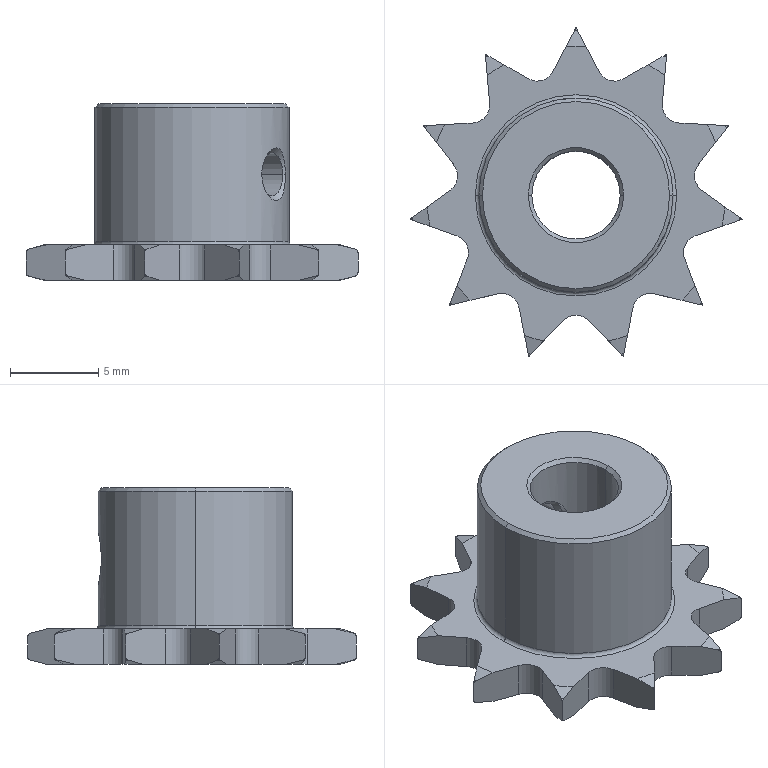Part | SolidWorks | features RevCut 2, ICE 1, Revolution 1 | 1 solid | 113 faces | box 18.807 x 18.615 x 10 mm | volume 909.903 mm3 | cone 36 | cylinder 28 | plane 25 | torus 24 | commonest cylinder face diameters 2 x14 3 x6 2.459 x4 5 x2 11 x2